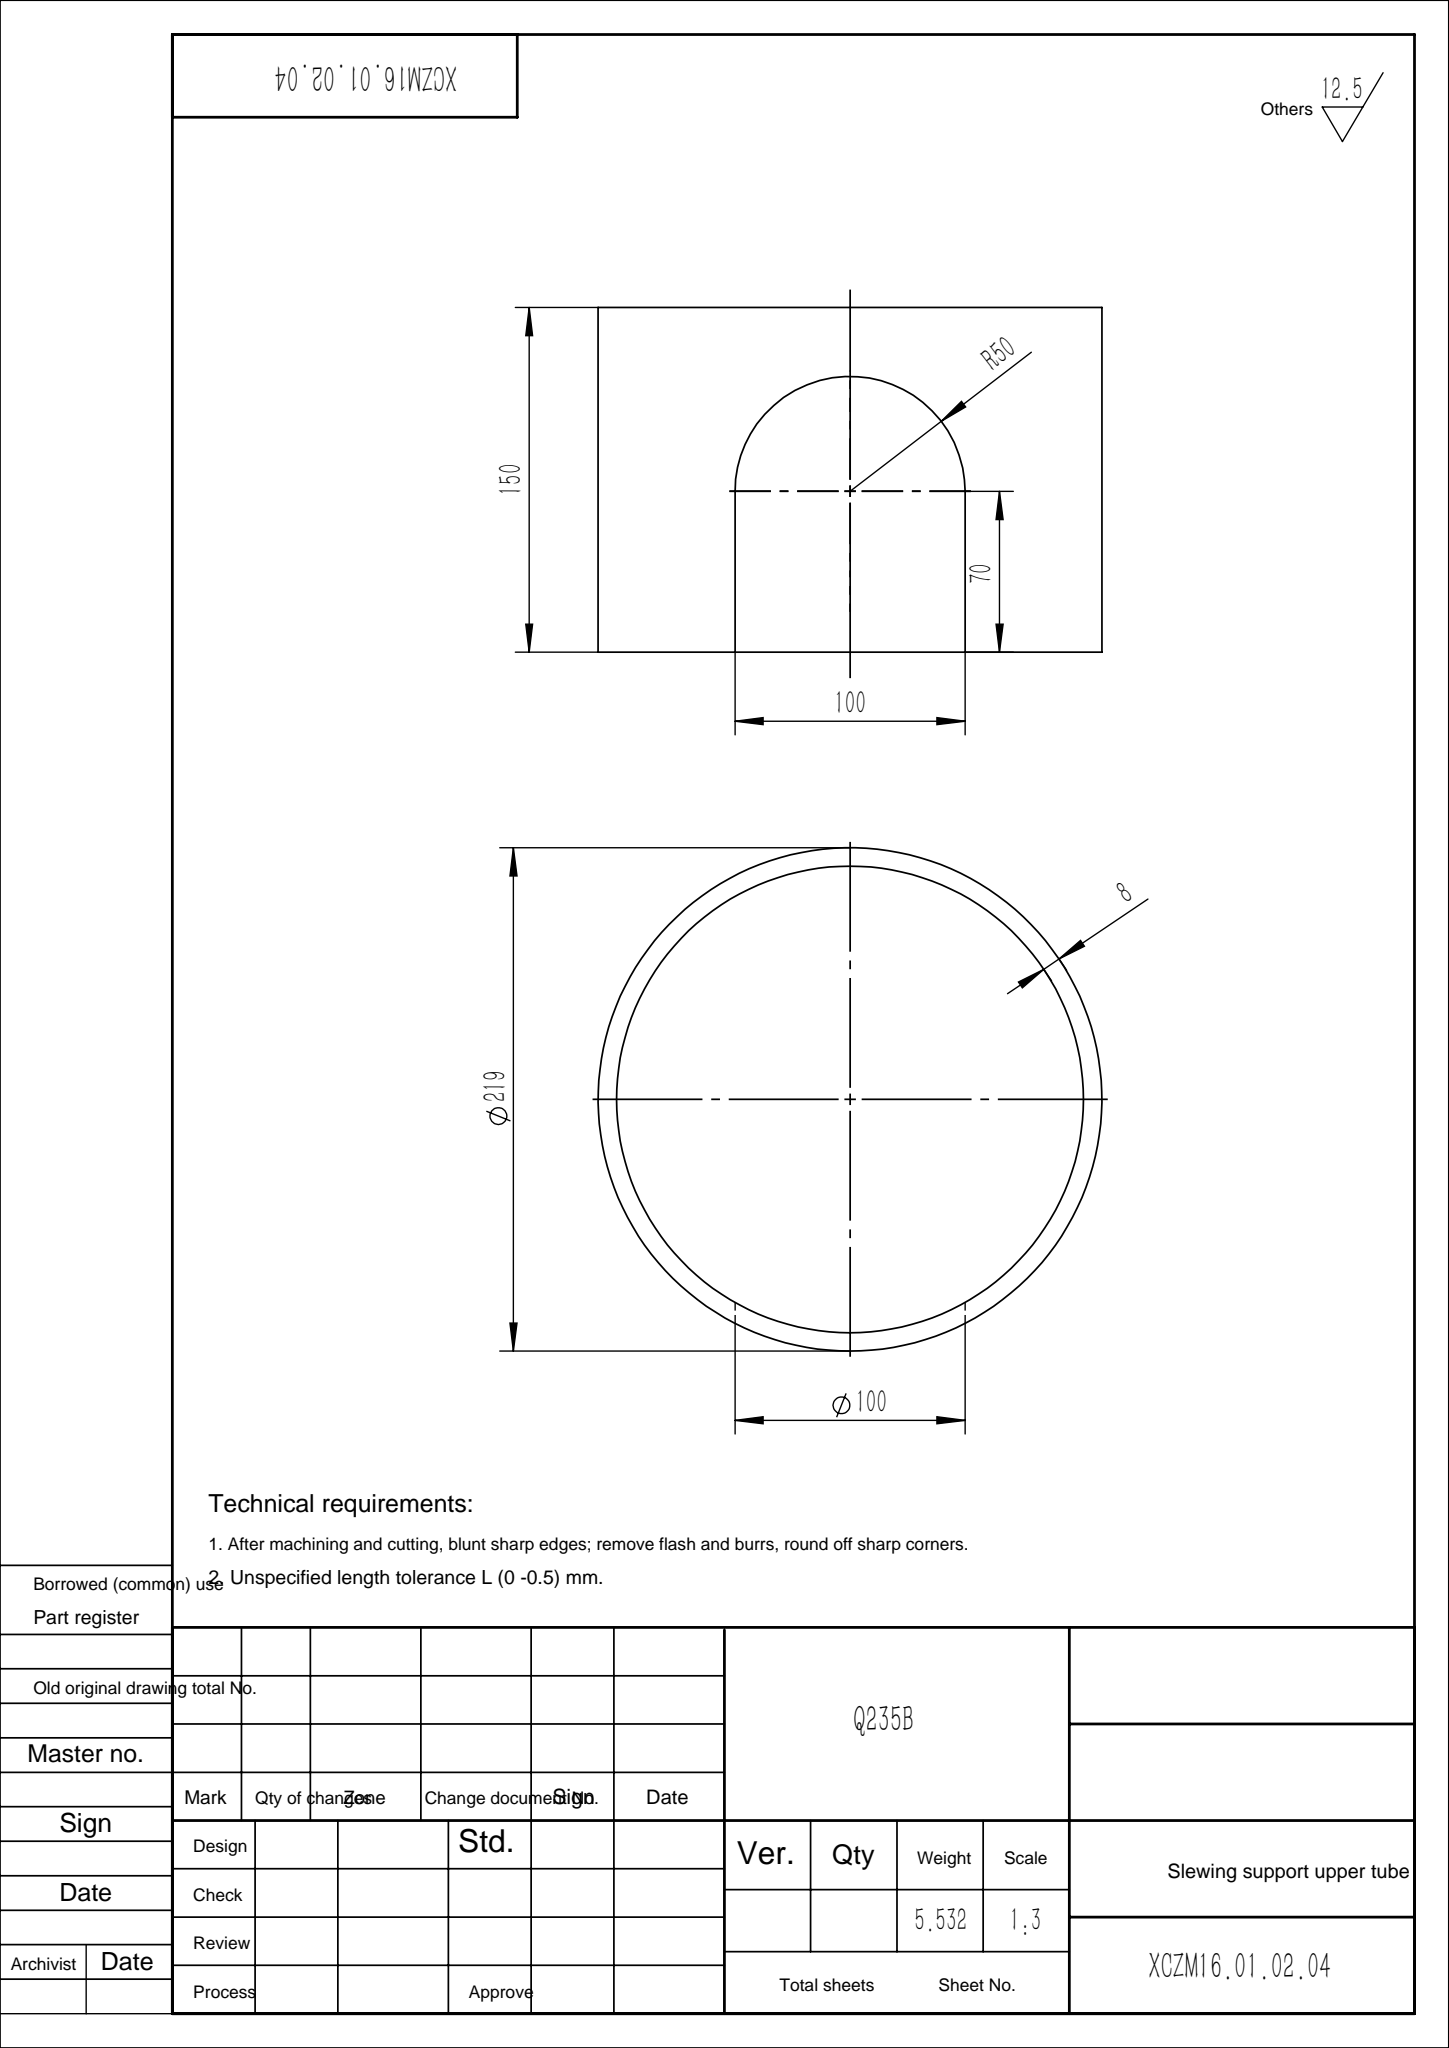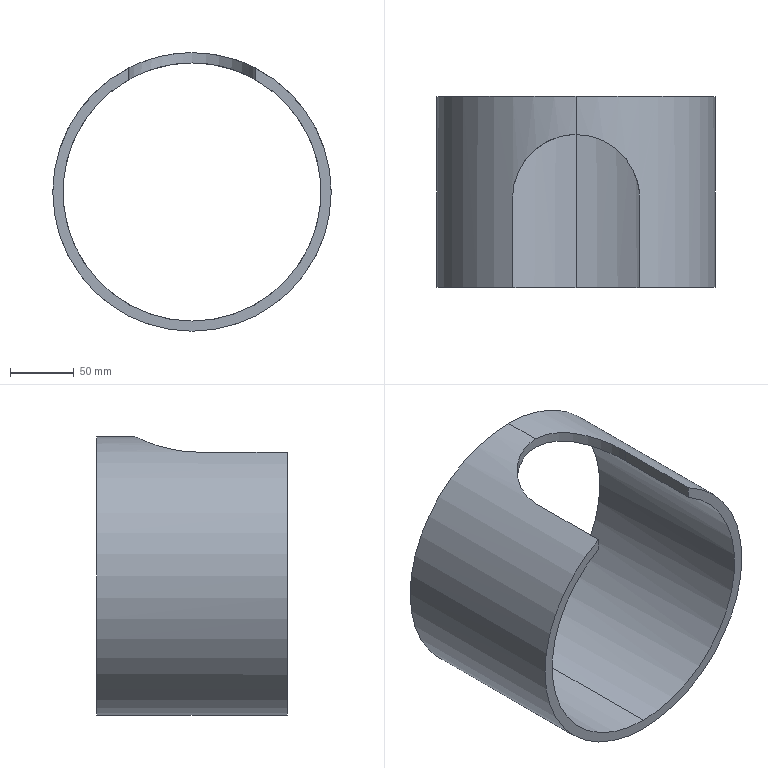Part | SolidWorks | features Extrusion 1, ICE 1 | 1 solid | 9 faces | box 219 x 150 x 219 mm | volume 704724 mm3 | cylinder 5 | plane 4 | commonest cylinder face diameters 203 x2 219 x2 100 x1
STEP:
#1=CARTESIAN_POINT('',(0.,150.,-101.5));
#2=VERTEX_POINT('',#1);
#3=CARTESIAN_POINT('',(0.,150.,101.5));
#4=VERTEX_POINT('',#3);
#5=CARTESIAN_POINT('',(0.,150.,0.));
#6=DIRECTION('',(0.,1.,0.));
#7=DIRECTION('',(0.,0.,1.));
#8=AXIS2_PLACEMENT_3D('',#5,#6,#7);
#9=CIRCLE('',#8,101.5);
#10=EDGE_CURVE('',#2,#4,#9,.T.);
#11=ORIENTED_EDGE('',*,*,#10,.T.);
#12=CARTESIAN_POINT('',(0.,120.,101.5));
#13=VERTEX_POINT('',#12);
#14=CARTESIAN_POINT('',(0.,150.,101.5));
#15=DIRECTION('',(0.,-1.,0.));
#16=VECTOR('',#15,1000.);
#17=LINE('',#14,#16);
#18=EDGE_CURVE('',#4,#13,#17,.T.);
#19=ORIENTED_EDGE('',*,*,#18,.T.);
#20=CARTESIAN_POINT('',(-50.,70.,88.33));
#21=VERTEX_POINT('',#20);
#22=CARTESIAN_POINT('',(-50.,70.,88.33));
#23=CARTESIAN_POINT('',(-50.,73.366,88.33));
#24=CARTESIAN_POINT('',(-49.664,76.662,88.523));
#25=CARTESIAN_POINT('',(-48.685,81.509,89.063));
#26=CARTESIAN_POINT('',(-48.279,83.109,89.284));
#27=CARTESIAN_POINT('',(-47.549,85.485,89.674));
#28=CARTESIAN_POINT('',(-47.285,86.272,89.813));
#29=CARTESIAN_POINT('',(-46.724,87.82,90.107));
#30=CARTESIAN_POINT('',(-46.426,88.583,90.261));
#31=CARTESIAN_POINT('',(-44.847,92.347,91.066));
#32=CARTESIAN_POINT('',(-43.31,95.195,91.817));
#33=CARTESIAN_POINT('',(-41.046,98.564,92.832));
#34=CARTESIAN_POINT('',(-40.574,99.23,93.039));
#35=CARTESIAN_POINT('',(-39.605,100.53,93.456));
#36=CARTESIAN_POINT('',(-39.107,101.166,93.665));
#37=CARTESIAN_POINT('',(-37.57,103.031,94.297));
#38=CARTESIAN_POINT('',(-36.491,104.22,94.721));
#39=CARTESIAN_POINT('',(-34.222,106.488,95.564));
#40=CARTESIAN_POINT('',(-33.033,107.569,95.983));
#41=CARTESIAN_POINT('',(-31.163,109.109,96.6));
#42=CARTESIAN_POINT('',(-30.525,109.609,96.804));
#43=CARTESIAN_POINT('',(-29.22,110.582,97.206));
#44=CARTESIAN_POINT('',(-28.553,111.054,97.404));
#45=CARTESIAN_POINT('',(-25.179,113.319,98.367));
#46=CARTESIAN_POINT('',(-22.33,114.855,99.061));
#47=CARTESIAN_POINT('',(-17.821,116.745,99.935));
#48=CARTESIAN_POINT('',(-16.278,117.305,100.199));
#49=CARTESIAN_POINT('',(-13.901,118.036,100.547));
#50=CARTESIAN_POINT('',(-13.095,118.262,100.655));
#51=CARTESIAN_POINT('',(-11.484,118.671,100.852));
#52=CARTESIAN_POINT('',(-10.675,118.854,100.94));
#53=CARTESIAN_POINT('',(-6.619,119.67,101.336));
#54=CARTESIAN_POINT('',(-3.331,120.,101.5));
#55=CARTESIAN_POINT('',(0.,120.,101.5));
#56=B_SPLINE_CURVE_WITH_KNOTS('',3,(#22,#23,#24,#25,#26,#27,#28,#29,#30,#31,#32,#33,#34,#35,#36,#37,#38,#39,#40,#41,#42,#43,#44,#45,#46,#47,#48,#49,#50,#51,#52,#53,#54,#55),.UNSPECIFIED.,.F.,.F.,(4,2,2,2,2,2,2,2,2,2,2,2,2,2,2,2,4),(0.,0.009938,0.01491,0.01739,0.01988,0.02981,0.0323,0.03478,0.03975,0.04472,0.0472,0.04969,0.05963,0.0646,0.06708,0.06956,0.0795),.UNSPECIFIED.);
#57=EDGE_CURVE('',#21,#13,#56,.T.);
#58=ORIENTED_EDGE('',*,*,#57,.F.);
#59=CARTESIAN_POINT('',(-50.,0.,88.33));
#60=VERTEX_POINT('',#59);
#61=CARTESIAN_POINT('',(-50.,150.,88.33));
#62=DIRECTION('',(0.,1.,0.));
#63=VECTOR('',#62,1000.);
#64=LINE('',#61,#63);
#65=EDGE_CURVE('',#60,#21,#64,.T.);
#66=ORIENTED_EDGE('',*,*,#65,.F.);
#67=CARTESIAN_POINT('',(0.,0.,-101.5));
#68=VERTEX_POINT('',#67);
#69=CARTESIAN_POINT('',(0.,0.,0.));
#70=DIRECTION('',(0.,1.,0.));
#71=DIRECTION('',(0.,0.,1.));
#72=AXIS2_PLACEMENT_3D('',#69,#70,#71);
#73=CIRCLE('',#72,101.5);
#74=EDGE_CURVE('',#68,#60,#73,.T.);
#75=ORIENTED_EDGE('',*,*,#74,.F.);
#76=CARTESIAN_POINT('',(0.,150.,-101.5));
#77=DIRECTION('',(0.,-1.,0.));
#78=VECTOR('',#77,1000.);
#79=LINE('',#76,#78);
#80=EDGE_CURVE('',#2,#68,#79,.T.);
#81=ORIENTED_EDGE('',*,*,#80,.F.);
#82=EDGE_LOOP('',(#11,#19,#58,#66,#75,#81));
#83=FACE_OUTER_BOUND('',#82,.T.);
#84=CARTESIAN_POINT('',(0.,150.,0.));
#85=DIRECTION('',(0.,-1.,0.));
#86=DIRECTION('',(0.,0.,-1.));
#87=AXIS2_PLACEMENT_3D('',#84,#85,#86);
#88=CYLINDRICAL_SURFACE('',#87,101.5);
#89=ADVANCED_FACE('',(#83),#88,.F.);
#90=CARTESIAN_POINT('',(0.,150.,109.5));
#91=VERTEX_POINT('',#90);
#92=CARTESIAN_POINT('',(0.,150.,-109.5));
#93=VERTEX_POINT('',#92);
#94=CARTESIAN_POINT('',(0.,150.,0.));
#95=DIRECTION('',(0.,1.,0.));
#96=DIRECTION('',(0.,0.,1.));
#97=AXIS2_PLACEMENT_3D('',#94,#95,#96);
#98=CIRCLE('',#97,109.5);
#99=EDGE_CURVE('',#91,#93,#98,.T.);
#100=ORIENTED_EDGE('',*,*,#99,.F.);
#101=CARTESIAN_POINT('',(0.,120.,109.5));
#102=VERTEX_POINT('',#101);
#103=CARTESIAN_POINT('',(0.,150.,109.5));
#104=DIRECTION('',(0.,-1.,0.));
#105=VECTOR('',#104,1000.);
#106=LINE('',#103,#105);
#107=EDGE_CURVE('',#91,#102,#106,.T.);
#108=ORIENTED_EDGE('',*,*,#107,.T.);
#109=CARTESIAN_POINT('',(50.,70.,97.418));
#110=VERTEX_POINT('',#109);
#111=CARTESIAN_POINT('',(0.,120.,109.5));
#112=CARTESIAN_POINT('',(0.8284,120.,109.5));
#113=CARTESIAN_POINT('',(1.659,119.979,109.491));
#114=CARTESIAN_POINT('',(3.326,119.896,109.453));
#115=CARTESIAN_POINT('',(4.162,119.833,109.424));
#116=CARTESIAN_POINT('',(6.647,119.584,109.311));
#117=CARTESIAN_POINT('',(8.281,119.337,109.198));
#118=CARTESIAN_POINT('',(11.507,118.686,108.906));
#119=CARTESIAN_POINT('',(13.099,118.282,108.725));
#120=CARTESIAN_POINT('',(15.456,117.558,108.407));
#121=CARTESIAN_POINT('',(16.236,117.298,108.292));
#122=CARTESIAN_POINT('',(17.786,116.737,108.049));
#123=CARTESIAN_POINT('',(18.558,116.436,107.919));
#124=CARTESIAN_POINT('',(22.355,114.845,107.238));
#125=CARTESIAN_POINT('',(25.209,113.301,106.595));
#126=CARTESIAN_POINT('',(29.239,110.592,105.533));
#127=CARTESIAN_POINT('',(30.541,109.622,105.163));
#128=CARTESIAN_POINT('',(33.053,107.552,104.4));
#129=CARTESIAN_POINT('',(34.248,106.465,104.013));
#130=CARTESIAN_POINT('',(37.657,103.05,102.849));
#131=CARTESIAN_POINT('',(39.698,100.571,102.069));
#132=CARTESIAN_POINT('',(41.96,97.203,101.143));
#133=CARTESIAN_POINT('',(42.399,96.514,100.959));
#134=CARTESIAN_POINT('',(43.241,95.118,100.602));
#135=CARTESIAN_POINT('',(43.644,94.411,100.427));
#136=CARTESIAN_POINT('',(44.797,92.267,99.921));
#137=CARTESIAN_POINT('',(45.495,90.805,99.604));
#138=CARTESIAN_POINT('',(46.747,87.815,99.023));
#139=CARTESIAN_POINT('',(47.301,86.287,98.758));
#140=CARTESIAN_POINT('',(48.265,83.16,98.291));
#141=CARTESIAN_POINT('',(48.674,81.56,98.088));
#142=CARTESIAN_POINT('',(49.666,76.66,97.591));
#143=CARTESIAN_POINT('',(50.,73.352,97.418));
#144=CARTESIAN_POINT('',(50.,70.,97.418));
#145=B_SPLINE_CURVE_WITH_KNOTS('',3,(#111,#112,#113,#114,#115,#116,#117,#118,#119,#120,#121,#122,#123,#124,#125,#126,#127,#128,#129,#130,#131,#132,#133,#134,#135,#136,#137,#138,#139,#140,#141,#142,#143,#144),.UNSPECIFIED.,.F.,.F.,(4,2,2,2,2,2,2,2,2,2,2,2,2,2,2,2,4),(0.0793,0.08177,0.08425,0.08919,0.09414,0.09661,0.09909,0.109,0.1139,0.1189,0.1288,0.1312,0.1337,0.1387,0.1436,0.1486,0.1585),.UNSPECIFIED.);
#146=EDGE_CURVE('',#102,#110,#145,.T.);
#147=ORIENTED_EDGE('',*,*,#146,.T.);
#148=CARTESIAN_POINT('',(50.,0.,97.418));
#149=VERTEX_POINT('',#148);
#150=CARTESIAN_POINT('',(50.,150.,97.418));
#151=DIRECTION('',(0.,-1.,0.));
#152=VECTOR('',#151,1000.);
#153=LINE('',#150,#152);
#154=EDGE_CURVE('',#110,#149,#153,.T.);
#155=ORIENTED_EDGE('',*,*,#154,.T.);
#156=CARTESIAN_POINT('',(0.,0.,-109.5));
#157=VERTEX_POINT('',#156);
#158=CARTESIAN_POINT('',(0.,0.,0.));
#159=DIRECTION('',(0.,1.,0.));
#160=DIRECTION('',(0.,0.,1.));
#161=AXIS2_PLACEMENT_3D('',#158,#159,#160);
#162=CIRCLE('',#161,109.5);
#163=EDGE_CURVE('',#149,#157,#162,.T.);
#164=ORIENTED_EDGE('',*,*,#163,.T.);
#165=CARTESIAN_POINT('',(0.,150.,-109.5));
#166=DIRECTION('',(0.,-1.,0.));
#167=VECTOR('',#166,1000.);
#168=LINE('',#165,#167);
#169=EDGE_CURVE('',#93,#157,#168,.T.);
#170=ORIENTED_EDGE('',*,*,#169,.F.);
#171=EDGE_LOOP('',(#100,#108,#147,#155,#164,#170));
#172=FACE_OUTER_BOUND('',#171,.T.);
#173=CARTESIAN_POINT('',(0.,150.,0.));
#174=DIRECTION('',(0.,-1.,0.));
#175=DIRECTION('',(0.,0.,-1.));
#176=AXIS2_PLACEMENT_3D('',#173,#174,#175);
#177=CYLINDRICAL_SURFACE('',#176,109.5);
#178=ADVANCED_FACE('',(#172),#177,.T.);
#179=CARTESIAN_POINT('',(50.,0.,88.33));
#180=VERTEX_POINT('',#179);
#181=CARTESIAN_POINT('',(50.,0.,109.501));
#182=DIRECTION('',(0.,0.,-1.));
#183=VECTOR('',#182,1000.);
#184=LINE('',#181,#183);
#185=EDGE_CURVE('',#149,#180,#184,.T.);
#186=ORIENTED_EDGE('',*,*,#185,.T.);
#187=CARTESIAN_POINT('',(0.,0.,0.));
#188=DIRECTION('',(0.,1.,0.));
#189=DIRECTION('',(0.,0.,1.));
#190=AXIS2_PLACEMENT_3D('',#187,#188,#189);
#191=CIRCLE('',#190,101.5);
#192=EDGE_CURVE('',#180,#68,#191,.T.);
#193=ORIENTED_EDGE('',*,*,#192,.T.);
#194=ORIENTED_EDGE('',*,*,#74,.T.);
#195=CARTESIAN_POINT('',(-50.,0.,97.418));
#196=VERTEX_POINT('',#195);
#197=CARTESIAN_POINT('',(-50.,0.,109.501));
#198=DIRECTION('',(0.,0.,-1.));
#199=VECTOR('',#198,1000.);
#200=LINE('',#197,#199);
#201=EDGE_CURVE('',#196,#60,#200,.T.);
#202=ORIENTED_EDGE('',*,*,#201,.F.);
#203=CARTESIAN_POINT('',(0.,0.,0.));
#204=DIRECTION('',(0.,1.,0.));
#205=DIRECTION('',(0.,0.,1.));
#206=AXIS2_PLACEMENT_3D('',#203,#204,#205);
#207=CIRCLE('',#206,109.5);
#208=EDGE_CURVE('',#157,#196,#207,.T.);
#209=ORIENTED_EDGE('',*,*,#208,.F.);
#210=ORIENTED_EDGE('',*,*,#163,.F.);
#211=EDGE_LOOP('',(#186,#193,#194,#202,#209,#210));
#212=FACE_OUTER_BOUND('',#211,.T.);
#213=CARTESIAN_POINT('',(0.,0.,0.));
#214=DIRECTION('',(0.,1.,0.));
#215=DIRECTION('',(0.,0.,1.));
#216=AXIS2_PLACEMENT_3D('',#213,#214,#215);
#217=PLANE('',#216);
#218=ADVANCED_FACE('',(#212),#217,.F.);
#219=ORIENTED_EDGE('',*,*,#107,.F.);
#220=CARTESIAN_POINT('',(0.,150.,0.));
#221=DIRECTION('',(0.,1.,0.));
#222=DIRECTION('',(0.,0.,1.));
#223=AXIS2_PLACEMENT_3D('',#220,#221,#222);
#224=CIRCLE('',#223,109.5);
#225=EDGE_CURVE('',#93,#91,#224,.T.);
#226=ORIENTED_EDGE('',*,*,#225,.F.);
#227=ORIENTED_EDGE('',*,*,#169,.T.);
#228=ORIENTED_EDGE('',*,*,#208,.T.);
#229=CARTESIAN_POINT('',(-50.,70.,97.418));
#230=VERTEX_POINT('',#229);
#231=CARTESIAN_POINT('',(-50.,150.,97.418));
#232=DIRECTION('',(0.,1.,0.));
#233=VECTOR('',#232,1000.);
#234=LINE('',#231,#233);
#235=EDGE_CURVE('',#196,#230,#234,.T.);
#236=ORIENTED_EDGE('',*,*,#235,.T.);
#237=CARTESIAN_POINT('',(-50.,70.,97.418));
#238=CARTESIAN_POINT('',(-50.,73.356,97.418));
#239=CARTESIAN_POINT('',(-49.666,76.645,97.591));
#240=CARTESIAN_POINT('',(-48.691,81.485,98.079));
#241=CARTESIAN_POINT('',(-48.286,83.083,98.28));
#242=CARTESIAN_POINT('',(-47.558,85.456,98.633));
#243=CARTESIAN_POINT('',(-47.295,86.243,98.76));
#244=CARTESIAN_POINT('',(-46.735,87.792,99.026));
#245=CARTESIAN_POINT('',(-46.436,88.556,99.167));
#246=CARTESIAN_POINT('',(-44.859,92.324,99.899));
#247=CARTESIAN_POINT('',(-43.321,95.176,100.585));
#248=CARTESIAN_POINT('',(-41.055,98.55,101.513));
#249=CARTESIAN_POINT('',(-40.584,99.217,101.703));
#250=CARTESIAN_POINT('',(-39.611,100.522,102.086));
#251=CARTESIAN_POINT('',(-39.111,101.16,102.278));
#252=CARTESIAN_POINT('',(-37.57,103.032,102.859));
#253=CARTESIAN_POINT('',(-36.488,104.223,103.249));
#254=CARTESIAN_POINT('',(-34.213,106.497,104.025));
#255=CARTESIAN_POINT('',(-33.021,107.579,104.41));
#256=CARTESIAN_POINT('',(-31.149,109.12,104.978));
#257=CARTESIAN_POINT('',(-30.51,109.62,105.166));
#258=CARTESIAN_POINT('',(-29.204,110.593,105.536));
#259=CARTESIAN_POINT('',(-28.535,111.066,105.719));
#260=CARTESIAN_POINT('',(-25.151,113.337,106.609));
#261=CARTESIAN_POINT('',(-22.296,114.872,107.249));
#262=CARTESIAN_POINT('',(-17.788,116.757,108.056));
#263=CARTESIAN_POINT('',(-16.247,117.316,108.3));
#264=CARTESIAN_POINT('',(-13.875,118.043,108.62));
#265=CARTESIAN_POINT('',(-13.072,118.268,108.72));
#266=CARTESIAN_POINT('',(-11.46,118.676,108.902));
#267=CARTESIAN_POINT('',(-10.652,118.859,108.984));
#268=CARTESIAN_POINT('',(-6.6,119.673,109.349));
#269=CARTESIAN_POINT('',(-3.319,120.,109.5));
#270=CARTESIAN_POINT('',(0.,120.,109.5));
#271=B_SPLINE_CURVE_WITH_KNOTS('',3,(#237,#238,#239,#240,#241,#242,#243,#244,#245,#246,#247,#248,#249,#250,#251,#252,#253,#254,#255,#256,#257,#258,#259,#260,#261,#262,#263,#264,#265,#266,#267,#268,#269,#270),.UNSPECIFIED.,.F.,.F.,(4,2,2,2,2,2,2,2,2,2,2,2,2,2,2,2,4),(0.,0.009912,0.01487,0.01735,0.01982,0.02974,0.03221,0.03469,0.03965,0.04461,0.04708,0.04956,0.05947,0.06443,0.06691,0.06939,0.0793),.UNSPECIFIED.);
#272=EDGE_CURVE('',#230,#102,#271,.T.);
#273=ORIENTED_EDGE('',*,*,#272,.T.);
#274=EDGE_LOOP('',(#219,#226,#227,#228,#236,#273));
#275=FACE_OUTER_BOUND('',#274,.T.);
#276=CARTESIAN_POINT('',(0.,150.,0.));
#277=DIRECTION('',(0.,-1.,0.));
#278=DIRECTION('',(0.,0.,-1.));
#279=AXIS2_PLACEMENT_3D('',#276,#277,#278);
#280=CYLINDRICAL_SURFACE('',#279,109.5);
#281=ADVANCED_FACE('',(#275),#280,.T.);
#282=ORIENTED_EDGE('',*,*,#18,.F.);
#283=CARTESIAN_POINT('',(0.,150.,0.));
#284=DIRECTION('',(0.,1.,0.));
#285=DIRECTION('',(0.,0.,1.));
#286=AXIS2_PLACEMENT_3D('',#283,#284,#285);
#287=CIRCLE('',#286,101.5);
#288=EDGE_CURVE('',#4,#2,#287,.T.);
#289=ORIENTED_EDGE('',*,*,#288,.T.);
#290=ORIENTED_EDGE('',*,*,#80,.T.);
#291=ORIENTED_EDGE('',*,*,#192,.F.);
#292=CARTESIAN_POINT('',(50.,70.,88.33));
#293=VERTEX_POINT('',#292);
#294=CARTESIAN_POINT('',(50.,150.,88.33));
#295=DIRECTION('',(0.,-1.,0.));
#296=VECTOR('',#295,1000.);
#297=LINE('',#294,#296);
#298=EDGE_CURVE('',#293,#180,#297,.T.);
#299=ORIENTED_EDGE('',*,*,#298,.F.);
#300=CARTESIAN_POINT('',(0.,120.,101.5));
#301=CARTESIAN_POINT('',(0.8312,120.,101.5));
#302=CARTESIAN_POINT('',(1.665,119.979,101.49));
#303=CARTESIAN_POINT('',(3.339,119.895,101.449));
#304=CARTESIAN_POINT('',(4.176,119.832,101.417));
#305=CARTESIAN_POINT('',(6.663,119.582,101.295));
#306=CARTESIAN_POINT('',(8.3,119.334,101.173));
#307=CARTESIAN_POINT('',(11.532,118.68,100.856));
#308=CARTESIAN_POINT('',(13.127,118.274,100.66));
#309=CARTESIAN_POINT('',(15.489,117.548,100.314));
#310=CARTESIAN_POINT('',(16.271,117.286,100.19));
#311=CARTESIAN_POINT('',(17.825,116.722,99.926));
#312=CARTESIAN_POINT('',(18.596,116.42,99.785));
#313=CARTESIAN_POINT('',(22.387,114.829,99.049));
#314=CARTESIAN_POINT('',(25.238,113.284,98.352));
#315=CARTESIAN_POINT('',(28.594,111.025,97.392));
#316=CARTESIAN_POINT('',(29.255,110.556,97.195));
#317=CARTESIAN_POINT('',(30.555,109.586,96.794));
#318=CARTESIAN_POINT('',(31.196,109.083,96.589));
#319=CARTESIAN_POINT('',(33.071,107.536,95.97));
#320=CARTESIAN_POINT('',(34.26,106.453,95.551));
#321=CARTESIAN_POINT('',(37.658,103.048,94.287));
#322=CARTESIAN_POINT('',(39.696,100.574,93.437));
#323=CARTESIAN_POINT('',(41.959,97.205,92.423));
#324=CARTESIAN_POINT('',(42.397,96.517,92.222));
#325=CARTESIAN_POINT('',(43.235,95.128,91.833));
#326=CARTESIAN_POINT('',(43.636,94.424,91.642));
#327=CARTESIAN_POINT('',(44.786,92.289,91.089));
#328=CARTESIAN_POINT('',(45.483,90.831,90.742));
#329=CARTESIAN_POINT('',(46.736,87.844,90.103));
#330=CARTESIAN_POINT('',(47.292,86.316,89.811));
#331=CARTESIAN_POINT('',(48.017,83.967,89.424));
#332=CARTESIAN_POINT('',(48.24,83.174,89.304));
#333=CARTESIAN_POINT('',(48.65,81.57,89.081));
#334=CARTESIAN_POINT('',(48.837,80.755,88.979));
#335=CARTESIAN_POINT('',(49.665,76.674,88.523));
#336=CARTESIAN_POINT('',(50.,73.361,88.33));
#337=CARTESIAN_POINT('',(50.,70.,88.33));
#338=B_SPLINE_CURVE_WITH_KNOTS('',3,(#300,#301,#302,#303,#304,#305,#306,#307,#308,#309,#310,#311,#312,#313,#314,#315,#316,#317,#318,#319,#320,#321,#322,#323,#324,#325,#326,#327,#328,#329,#330,#331,#332,#333,#334,#335,#336,#337),.UNSPECIFIED.,.F.,.F.,(4,2,2,2,2,2,2,2,2,2,2,2,2,2,2,2,2,2,4),(0.0795,0.08198,0.08446,0.08942,0.09438,0.09686,0.09934,0.1093,0.1117,0.1142,0.1192,0.1291,0.1316,0.1341,0.139,0.144,0.1465,0.1489,0.1589),.UNSPECIFIED.);
#339=EDGE_CURVE('',#13,#293,#338,.T.);
#340=ORIENTED_EDGE('',*,*,#339,.F.);
#341=EDGE_LOOP('',(#282,#289,#290,#291,#299,#340));
#342=FACE_OUTER_BOUND('',#341,.T.);
#343=CARTESIAN_POINT('',(0.,150.,0.));
#344=DIRECTION('',(0.,-1.,0.));
#345=DIRECTION('',(0.,0.,-1.));
#346=AXIS2_PLACEMENT_3D('',#343,#344,#345);
#347=CYLINDRICAL_SURFACE('',#346,101.5);
#348=ADVANCED_FACE('',(#342),#347,.F.);
#349=ORIENTED_EDGE('',*,*,#225,.T.);
#350=ORIENTED_EDGE('',*,*,#99,.T.);
#351=EDGE_LOOP('',(#349,#350));
#352=FACE_OUTER_BOUND('',#351,.T.);
#353=ORIENTED_EDGE('',*,*,#10,.F.);
#354=ORIENTED_EDGE('',*,*,#288,.F.);
#355=EDGE_LOOP('',(#353,#354));
#356=FACE_BOUND('',#355,.T.);
#357=CARTESIAN_POINT('',(0.,150.,0.));
#358=DIRECTION('',(0.,1.,0.));
#359=DIRECTION('',(0.,0.,1.));
#360=AXIS2_PLACEMENT_3D('',#357,#358,#359);
#361=PLANE('',#360);
#362=ADVANCED_FACE('',(#352,#356),#361,.T.);
#363=CARTESIAN_POINT('',(50.,70.,109.501));
#364=DIRECTION('',(0.,0.,-1.));
#365=VECTOR('',#364,1000.);
#366=LINE('',#363,#365);
#367=EDGE_CURVE('',#110,#293,#366,.T.);
#368=ORIENTED_EDGE('',*,*,#367,.T.);
#369=ORIENTED_EDGE('',*,*,#298,.T.);
#370=ORIENTED_EDGE('',*,*,#185,.F.);
#371=ORIENTED_EDGE('',*,*,#154,.F.);
#372=EDGE_LOOP('',(#368,#369,#370,#371));
#373=FACE_OUTER_BOUND('',#372,.T.);
#374=CARTESIAN_POINT('',(50.,0.,109.501));
#375=DIRECTION('',(-1.,0.,0.));
#376=DIRECTION('',(0.,0.,1.));
#377=AXIS2_PLACEMENT_3D('',#374,#375,#376);
#378=PLANE('',#377);
#379=ADVANCED_FACE('',(#373),#378,.T.);
#380=CARTESIAN_POINT('',(-50.,70.,109.501));
#381=DIRECTION('',(0.,0.,-1.));
#382=VECTOR('',#381,1000.);
#383=LINE('',#380,#382);
#384=EDGE_CURVE('',#230,#21,#383,.T.);
#385=ORIENTED_EDGE('',*,*,#384,.T.);
#386=ORIENTED_EDGE('',*,*,#57,.T.);
#387=ORIENTED_EDGE('',*,*,#339,.T.);
#388=ORIENTED_EDGE('',*,*,#367,.F.);
#389=ORIENTED_EDGE('',*,*,#146,.F.);
#390=ORIENTED_EDGE('',*,*,#272,.F.);
#391=EDGE_LOOP('',(#385,#386,#387,#388,#389,#390));
#392=FACE_OUTER_BOUND('',#391,.T.);
#393=CARTESIAN_POINT('',(0.,70.,109.501));
#394=DIRECTION('',(0.,0.,-1.));
#395=DIRECTION('',(-1.,0.,0.));
#396=AXIS2_PLACEMENT_3D('',#393,#394,#395);
#397=CYLINDRICAL_SURFACE('',#396,50.);
#398=ADVANCED_FACE('',(#392),#397,.F.);
#399=ORIENTED_EDGE('',*,*,#201,.T.);
#400=ORIENTED_EDGE('',*,*,#65,.T.);
#401=ORIENTED_EDGE('',*,*,#384,.F.);
#402=ORIENTED_EDGE('',*,*,#235,.F.);
#403=EDGE_LOOP('',(#399,#400,#401,#402));
#404=FACE_OUTER_BOUND('',#403,.T.);
#405=CARTESIAN_POINT('',(-50.,0.,109.501));
#406=DIRECTION('',(1.,0.,0.));
#407=DIRECTION('',(0.,0.,-1.));
#408=AXIS2_PLACEMENT_3D('',#405,#406,#407);
#409=PLANE('',#408);
#410=ADVANCED_FACE('',(#404),#409,.T.);
#411=CLOSED_SHELL('',(#89,#178,#218,#281,#348,#362,#379,#398,#410));
#412=MANIFOLD_SOLID_BREP('',#411);
#413=CARTESIAN_POINT('',(0.,0.,0.));
#414=DIRECTION('',(0.,0.,1.));
#415=DIRECTION('',(1.,0.,0.));
#416=AXIS2_PLACEMENT_3D('',#413,#414,#415);
#417=(LENGTH_UNIT()NAMED_UNIT(*)SI_UNIT(.MILLI.,.METRE.));
#418=UNCERTAINTY_MEASURE_WITH_UNIT(LENGTH_MEASURE(0.00001),#417,'','');
#419=(NAMED_UNIT(*)PLANE_ANGLE_UNIT()SI_UNIT($,.RADIAN.));
#420=(NAMED_UNIT(*)SI_UNIT($,.STERADIAN.)SOLID_ANGLE_UNIT());
#421=(GEOMETRIC_REPRESENTATION_CONTEXT(3)GLOBAL_UNCERTAINTY_ASSIGNED_CONTEXT((#418))GLOBAL_UNIT_ASSIGNED_CONTEXT((#417,#419,#420))REPRESENTATION_CONTEXT('',''));
#422=ADVANCED_BREP_SHAPE_REPRESENTATION('',(#412,#416),#421);